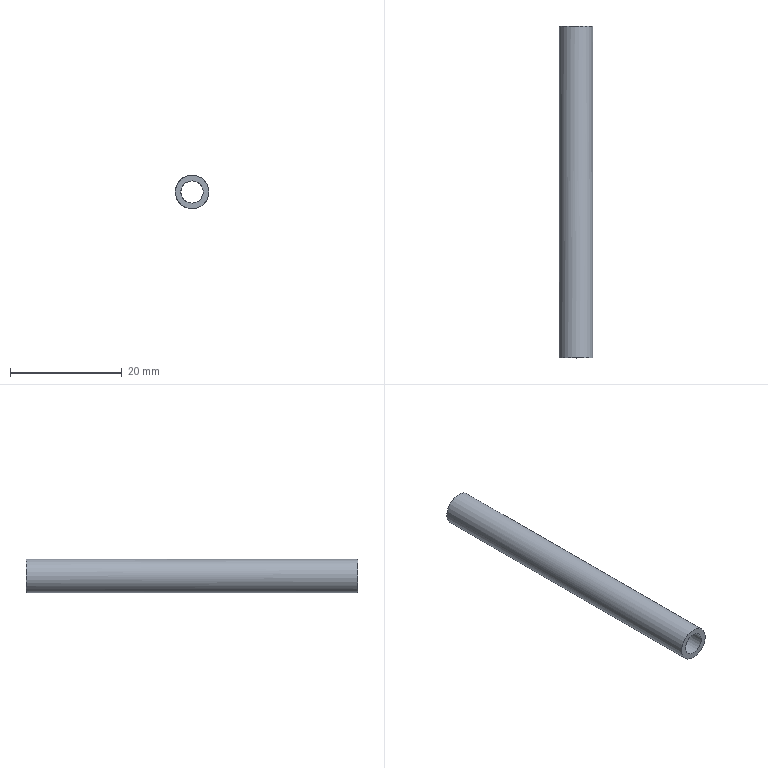Part | NX | features solid 2 | 1 solid | 4 faces | box 6 x 59.488 x 6 mm | volume 934.433 mm3 | cylinder 2 | plane 2 | commonest cylinder face diameters 4 x1 6 x1
STEP:
#1=CARTESIAN_POINT('',(271.,127.875,347.));
#2=VERTEX_POINT('',#1);
#3=CARTESIAN_POINT('',(273.,127.875,347.));
#4=DIRECTION('',(0.,1.,0.));
#5=DIRECTION('',(-1.,0.,0.));
#6=AXIS2_PLACEMENT_3D('',#3,#4,#5);
#7=CIRCLE('',#6,2.);
#8=EDGE_CURVE('',#2,#2,#7,.T.);
#9=ORIENTED_EDGE('',*,*,#8,.T.);
#10=EDGE_LOOP('',(#9));
#11=FACE_BOUND('',#10,.T.);
#12=CARTESIAN_POINT('',(273.,68.387,345.));
#13=VERTEX_POINT('',#12);
#14=CARTESIAN_POINT('',(273.,68.387,347.));
#15=DIRECTION('',(0.,-1.,0.));
#16=DIRECTION('',(0.,0.,-1.));
#17=AXIS2_PLACEMENT_3D('',#14,#15,#16);
#18=CIRCLE('',#17,2.);
#19=EDGE_CURVE('',#13,#13,#18,.T.);
#20=ORIENTED_EDGE('',*,*,#19,.T.);
#21=EDGE_LOOP('',(#20));
#22=FACE_BOUND('',#21,.T.);
#23=CARTESIAN_POINT('',(273.,228.824,347.));
#24=DIRECTION('',(0.,-1.,0.));
#25=DIRECTION('',(1.,0.,0.));
#26=AXIS2_PLACEMENT_3D('',#23,#24,#25);
#27=CYLINDRICAL_SURFACE('',#26,2.);
#28=ADVANCED_FACE('',(#11,#22),#27,.F.);
#29=CARTESIAN_POINT('',(270.,127.875,347.));
#30=VERTEX_POINT('',#29);
#31=CARTESIAN_POINT('',(273.,127.875,347.));
#32=DIRECTION('',(0.,1.,0.));
#33=DIRECTION('',(-1.,0.,0.));
#34=AXIS2_PLACEMENT_3D('',#31,#32,#33);
#35=CIRCLE('',#34,3.);
#36=EDGE_CURVE('',#30,#30,#35,.T.);
#37=ORIENTED_EDGE('',*,*,#36,.F.);
#38=EDGE_LOOP('',(#37));
#39=FACE_BOUND('',#38,.T.);
#40=CARTESIAN_POINT('',(273.,68.387,344.));
#41=VERTEX_POINT('',#40);
#42=CARTESIAN_POINT('',(273.,68.387,347.));
#43=DIRECTION('',(0.,-1.,0.));
#44=DIRECTION('',(0.,0.,-1.));
#45=AXIS2_PLACEMENT_3D('',#42,#43,#44);
#46=CIRCLE('',#45,3.);
#47=EDGE_CURVE('',#41,#41,#46,.T.);
#48=ORIENTED_EDGE('',*,*,#47,.F.);
#49=EDGE_LOOP('',(#48));
#50=FACE_BOUND('',#49,.T.);
#51=CARTESIAN_POINT('',(273.,228.824,347.));
#52=DIRECTION('',(0.,-1.,0.));
#53=DIRECTION('',(1.,0.,0.));
#54=AXIS2_PLACEMENT_3D('',#51,#52,#53);
#55=CYLINDRICAL_SURFACE('',#54,3.);
#56=ADVANCED_FACE('',(#39,#50),#55,.T.);
#57=ORIENTED_EDGE('',*,*,#8,.F.);
#58=EDGE_LOOP('',(#57));
#59=FACE_BOUND('',#58,.T.);
#60=ORIENTED_EDGE('',*,*,#36,.T.);
#61=EDGE_LOOP('',(#60));
#62=FACE_BOUND('',#61,.T.);
#63=CARTESIAN_POINT('',(312.83,127.875,185.));
#64=DIRECTION('',(0.,1.,0.));
#65=DIRECTION('',(-1.,0.,0.));
#66=AXIS2_PLACEMENT_3D('',#63,#64,#65);
#67=PLANE('',#66);
#68=ADVANCED_FACE('',(#59,#62),#67,.T.);
#69=ORIENTED_EDGE('',*,*,#19,.F.);
#70=EDGE_LOOP('',(#69));
#71=FACE_BOUND('',#70,.T.);
#72=ORIENTED_EDGE('',*,*,#47,.T.);
#73=EDGE_LOOP('',(#72));
#74=FACE_BOUND('',#73,.T.);
#75=CARTESIAN_POINT('',(367.131,68.387,203.));
#76=DIRECTION('',(0.,-1.,0.));
#77=DIRECTION('',(0.,0.,-1.));
#78=AXIS2_PLACEMENT_3D('',#75,#76,#77);
#79=PLANE('',#78);
#80=ADVANCED_FACE('',(#71,#74),#79,.T.);
#81=CLOSED_SHELL('',(#28,#56,#68,#80));
#82=MANIFOLD_SOLID_BREP('',#81);
#83=(LENGTH_UNIT()NAMED_UNIT(*)SI_UNIT(.MILLI.,.METRE.));
#84=UNCERTAINTY_MEASURE_WITH_UNIT(LENGTH_MEASURE(0.00001),#83,'','');
#85=(NAMED_UNIT(*)PLANE_ANGLE_UNIT()SI_UNIT($,.RADIAN.));
#86=(NAMED_UNIT(*)SI_UNIT($,.STERADIAN.)SOLID_ANGLE_UNIT());
#87=(GEOMETRIC_REPRESENTATION_CONTEXT(3)GLOBAL_UNCERTAINTY_ASSIGNED_CONTEXT((#84))GLOBAL_UNIT_ASSIGNED_CONTEXT((#83,#85,#86))REPRESENTATION_CONTEXT('',''));
#88=ADVANCED_BREP_SHAPE_REPRESENTATION('',(#82),#87);